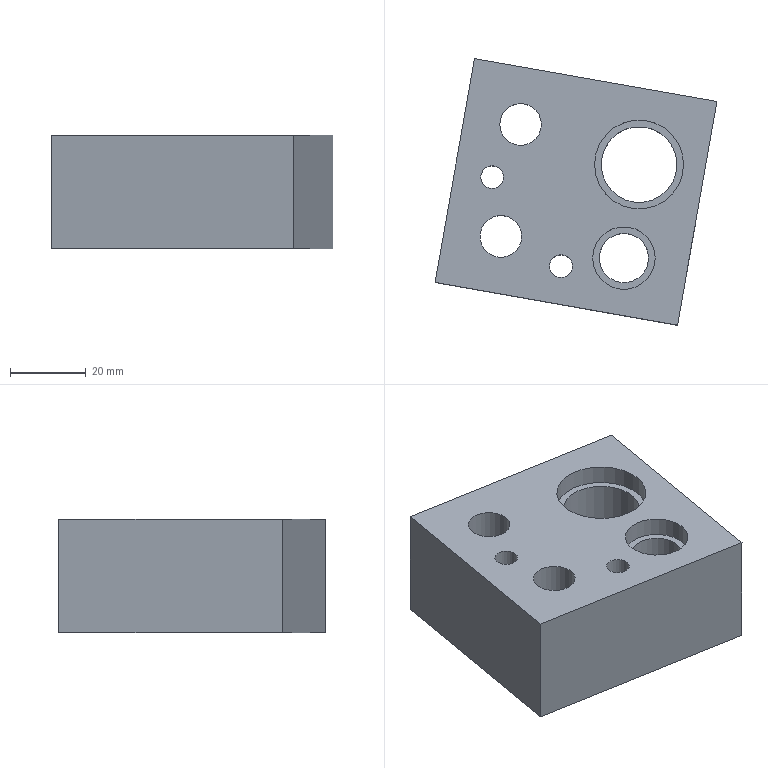Part | NX | features solid 2 | 1 solid | 20 faces | box 74.431 x 70.376 x 30 mm | volume 92025 mm3 | plane 10 | cylinder 10 | commonest cylinder face diameters 6 x2 11 x2 17 x2 13 x1 16.5 x1 20 x1
STEP:
#1=CARTESIAN_POINT('',(471.302,165.949,33.192));
#2=VERTEX_POINT('',#1);
#3=CARTESIAN_POINT('',(461.302,165.949,33.192));
#4=DIRECTION('',(0.000000502,0.000000149,1.));
#5=DIRECTION('',(1.,-0.000001668,-0.000000502));
#6=AXIS2_PLACEMENT_3D('',#3,#4,#5);
#7=CIRCLE('',#6,10.);
#8=EDGE_CURVE('',#2,#2,#7,.F.);
#9=ORIENTED_EDGE('',*,*,#8,.F.);
#10=EDGE_LOOP('',(#9));
#11=FACE_BOUND('',#10,.T.);
#12=CARTESIAN_POINT('',(416.303,147.002,33.192));
#13=VERTEX_POINT('',#12);
#14=CARTESIAN_POINT('',(424.803,147.002,33.192));
#15=DIRECTION('',(-0.000000502,-0.000000149,-1.));
#16=DIRECTION('',(-1.,0.000001668,0.000000502));
#17=AXIS2_PLACEMENT_3D('',#14,#15,#16);
#18=CIRCLE('',#17,8.5);
#19=EDGE_CURVE('',#13,#13,#18,.T.);
#20=ORIENTED_EDGE('',*,*,#19,.F.);
#21=EDGE_LOOP('',(#20));
#22=FACE_BOUND('',#21,.T.);
#23=CARTESIAN_POINT('',(421.512,176.546,33.192));
#24=VERTEX_POINT('',#23);
#25=CARTESIAN_POINT('',(430.012,176.546,33.192));
#26=DIRECTION('',(-0.000000502,-0.000000149,-1.));
#27=DIRECTION('',(-1.,0.000001668,0.000000502));
#28=AXIS2_PLACEMENT_3D('',#25,#26,#27);
#29=CIRCLE('',#28,8.5);
#30=EDGE_CURVE('',#24,#24,#29,.T.);
#31=ORIENTED_EDGE('',*,*,#30,.F.);
#32=EDGE_LOOP('',(#31));
#33=FACE_BOUND('',#32,.T.);
#34=CARTESIAN_POINT('',(407.426,134.834,33.192));
#35=VERTEX_POINT('',#34);
#36=CARTESIAN_POINT('',(417.845,193.923,33.192));
#37=VERTEX_POINT('',#36);
#38=CARTESIAN_POINT('',(418.713,198.847,33.192));
#39=DIRECTION('',(0.1736,0.9848,-0.000000234));
#40=VECTOR('',#39,1000.);
#41=LINE('',#38,#40);
#42=EDGE_CURVE('',#35,#37,#41,.T.);
#43=ORIENTED_EDGE('',*,*,#42,.T.);
#44=CARTESIAN_POINT('',(481.857,182.635,33.192));
#45=VERTEX_POINT('',#44);
#46=CARTESIAN_POINT('',(415.875,194.27,33.192));
#47=DIRECTION('',(0.9848,-0.1736,-0.000000468));
#48=VECTOR('',#47,1000.);
#49=LINE('',#46,#48);
#50=EDGE_CURVE('',#37,#45,#49,.T.);
#51=ORIENTED_EDGE('',*,*,#50,.T.);
#52=CARTESIAN_POINT('',(471.438,123.547,33.192));
#53=VERTEX_POINT('',#52);
#54=CARTESIAN_POINT('',(482.726,187.559,33.192));
#55=DIRECTION('',(-0.1736,-0.9848,0.000000234));
#56=VECTOR('',#55,1000.);
#57=LINE('',#54,#56);
#58=EDGE_CURVE('',#45,#53,#57,.T.);
#59=ORIENTED_EDGE('',*,*,#58,.T.);
#60=CARTESIAN_POINT('',(405.456,135.181,33.192));
#61=DIRECTION('',(-0.9848,0.1736,0.000000468));
#62=VECTOR('',#61,1000.);
#63=LINE('',#60,#62);
#64=EDGE_CURVE('',#53,#35,#63,.T.);
#65=ORIENTED_EDGE('',*,*,#64,.T.);
#66=EDGE_LOOP('',(#43,#51,#59,#65));
#67=FACE_BOUND('',#66,.T.);
#68=CARTESIAN_POINT('',(463.801,141.271,33.192));
#69=VERTEX_POINT('',#68);
#70=CARTESIAN_POINT('',(457.301,141.271,33.192));
#71=DIRECTION('',(0.000000502,0.000000149,1.));
#72=DIRECTION('',(1.,-0.000001668,-0.000000502));
#73=AXIS2_PLACEMENT_3D('',#70,#71,#72);
#74=CIRCLE('',#73,6.5);
#75=EDGE_CURVE('',#69,#69,#74,.F.);
#76=ORIENTED_EDGE('',*,*,#75,.F.);
#77=EDGE_LOOP('',(#76));
#78=FACE_BOUND('',#77,.T.);
#79=CARTESIAN_POINT('',(425.484,162.642,33.192));
#80=VERTEX_POINT('',#79);
#81=CARTESIAN_POINT('',(422.484,162.642,33.192));
#82=DIRECTION('',(0.000000502,0.000000149,1.));
#83=DIRECTION('',(1.,0.,-0.000000502));
#84=AXIS2_PLACEMENT_3D('',#81,#82,#83);
#85=CIRCLE('',#84,3.);
#86=EDGE_CURVE('',#80,#80,#85,.F.);
#87=ORIENTED_EDGE('',*,*,#86,.F.);
#88=EDGE_LOOP('',(#87));
#89=FACE_BOUND('',#88,.T.);
#90=CARTESIAN_POINT('',(443.676,139.125,33.192));
#91=VERTEX_POINT('',#90);
#92=CARTESIAN_POINT('',(440.676,139.125,33.192));
#93=DIRECTION('',(0.000000502,0.000000149,1.));
#94=DIRECTION('',(1.,0.,-0.000000502));
#95=AXIS2_PLACEMENT_3D('',#92,#93,#94);
#96=CIRCLE('',#95,3.);
#97=EDGE_CURVE('',#91,#91,#96,.F.);
#98=ORIENTED_EDGE('',*,*,#97,.F.);
#99=EDGE_LOOP('',(#98));
#100=FACE_BOUND('',#99,.T.);
#101=CARTESIAN_POINT('',(416.744,199.194,33.192));
#102=DIRECTION('',(-0.000000502,-0.000000149,-1.));
#103=DIRECTION('',(0.9848,-0.1736,-0.000000468));
#104=AXIS2_PLACEMENT_3D('',#101,#102,#103);
#105=PLANE('',#104);
#106=ADVANCED_FACE('',(#11,#22,#33,#67,#78,#89,#100),#105,.T.);
#107=CARTESIAN_POINT('',(443.676,139.125,63.192));
#108=VERTEX_POINT('',#107);
#109=CARTESIAN_POINT('',(440.676,139.125,63.192));
#110=DIRECTION('',(0.000000502,0.000000149,1.));
#111=DIRECTION('',(1.,-0.000001668,-0.000000502));
#112=AXIS2_PLACEMENT_3D('',#109,#110,#111);
#113=CIRCLE('',#112,3.);
#114=EDGE_CURVE('',#108,#108,#113,.F.);
#115=ORIENTED_EDGE('',*,*,#114,.T.);
#116=EDGE_LOOP('',(#115));
#117=FACE_BOUND('',#116,.T.);
#118=CARTESIAN_POINT('',(425.484,162.642,63.192));
#119=VERTEX_POINT('',#118);
#120=CARTESIAN_POINT('',(422.484,162.642,63.192));
#121=DIRECTION('',(0.000000502,0.000000149,1.));
#122=DIRECTION('',(1.,-0.000001668,-0.000000502));
#123=AXIS2_PLACEMENT_3D('',#120,#121,#122);
#124=CIRCLE('',#123,3.);
#125=EDGE_CURVE('',#119,#119,#124,.F.);
#126=ORIENTED_EDGE('',*,*,#125,.T.);
#127=EDGE_LOOP('',(#126));
#128=FACE_BOUND('',#127,.T.);
#129=CARTESIAN_POINT('',(473.052,165.949,63.192));
#130=VERTEX_POINT('',#129);
#131=CARTESIAN_POINT('',(461.302,165.949,63.192));
#132=DIRECTION('',(0.000000502,0.000000149,1.));
#133=DIRECTION('',(1.,-0.000001668,-0.000000502));
#134=AXIS2_PLACEMENT_3D('',#131,#132,#133);
#135=CIRCLE('',#134,11.75);
#136=EDGE_CURVE('',#130,#130,#135,.T.);
#137=ORIENTED_EDGE('',*,*,#136,.F.);
#138=EDGE_LOOP('',(#137));
#139=FACE_BOUND('',#138,.T.);
#140=CARTESIAN_POINT('',(430.303,147.002,63.192));
#141=VERTEX_POINT('',#140);
#142=CARTESIAN_POINT('',(424.803,147.002,63.192));
#143=DIRECTION('',(0.000000502,0.000000149,1.));
#144=DIRECTION('',(1.,-0.000001668,-0.000000502));
#145=AXIS2_PLACEMENT_3D('',#142,#143,#144);
#146=CIRCLE('',#145,5.5);
#147=EDGE_CURVE('',#141,#141,#146,.F.);
#148=ORIENTED_EDGE('',*,*,#147,.T.);
#149=EDGE_LOOP('',(#148));
#150=FACE_BOUND('',#149,.T.);
#151=CARTESIAN_POINT('',(435.512,176.546,63.192));
#152=VERTEX_POINT('',#151);
#153=CARTESIAN_POINT('',(430.012,176.546,63.192));
#154=DIRECTION('',(0.000000502,0.000000149,1.));
#155=DIRECTION('',(1.,-0.000001668,-0.000000502));
#156=AXIS2_PLACEMENT_3D('',#153,#154,#155);
#157=CIRCLE('',#156,5.5);
#158=EDGE_CURVE('',#152,#152,#157,.F.);
#159=ORIENTED_EDGE('',*,*,#158,.T.);
#160=EDGE_LOOP('',(#159));
#161=FACE_BOUND('',#160,.T.);
#162=CARTESIAN_POINT('',(407.426,134.834,63.192));
#163=VERTEX_POINT('',#162);
#164=CARTESIAN_POINT('',(471.438,123.547,63.192));
#165=VERTEX_POINT('',#164);
#166=CARTESIAN_POINT('',(405.456,135.181,63.192));
#167=DIRECTION('',(-0.9848,0.1736,0.000000468));
#168=VECTOR('',#167,1000.);
#169=LINE('',#166,#168);
#170=EDGE_CURVE('',#163,#165,#169,.F.);
#171=ORIENTED_EDGE('',*,*,#170,.T.);
#172=CARTESIAN_POINT('',(481.857,182.635,63.192));
#173=VERTEX_POINT('',#172);
#174=CARTESIAN_POINT('',(482.726,187.559,63.192));
#175=DIRECTION('',(-0.1736,-0.9848,0.000000234));
#176=VECTOR('',#175,1000.);
#177=LINE('',#174,#176);
#178=EDGE_CURVE('',#165,#173,#177,.F.);
#179=ORIENTED_EDGE('',*,*,#178,.T.);
#180=CARTESIAN_POINT('',(417.845,193.923,63.192));
#181=VERTEX_POINT('',#180);
#182=CARTESIAN_POINT('',(415.875,194.27,63.192));
#183=DIRECTION('',(0.9848,-0.1736,-0.000000468));
#184=VECTOR('',#183,1000.);
#185=LINE('',#182,#184);
#186=EDGE_CURVE('',#173,#181,#185,.F.);
#187=ORIENTED_EDGE('',*,*,#186,.T.);
#188=CARTESIAN_POINT('',(418.713,198.847,63.192));
#189=DIRECTION('',(0.1736,0.9848,-0.000000234));
#190=VECTOR('',#189,1000.);
#191=LINE('',#188,#190);
#192=EDGE_CURVE('',#181,#163,#191,.F.);
#193=ORIENTED_EDGE('',*,*,#192,.T.);
#194=EDGE_LOOP('',(#171,#179,#187,#193));
#195=FACE_BOUND('',#194,.T.);
#196=CARTESIAN_POINT('',(465.551,141.271,63.192));
#197=VERTEX_POINT('',#196);
#198=CARTESIAN_POINT('',(457.301,141.271,63.192));
#199=DIRECTION('',(0.000000502,0.000000149,1.));
#200=DIRECTION('',(1.,-0.000001668,-0.000000502));
#201=AXIS2_PLACEMENT_3D('',#198,#199,#200);
#202=CIRCLE('',#201,8.25);
#203=EDGE_CURVE('',#197,#197,#202,.T.);
#204=ORIENTED_EDGE('',*,*,#203,.F.);
#205=EDGE_LOOP('',(#204));
#206=FACE_BOUND('',#205,.T.);
#207=CARTESIAN_POINT('',(486.873,147.734,63.192));
#208=DIRECTION('',(-0.000000502,-0.000000149,-1.));
#209=DIRECTION('',(0.9848,-0.1736,-0.000000468));
#210=AXIS2_PLACEMENT_3D('',#207,#208,#209);
#211=PLANE('',#210);
#212=ADVANCED_FACE('',(#117,#128,#139,#150,#161,#195,#206),#211,.F.);
#213=CARTESIAN_POINT('',(407.426,134.834,63.192));
#214=DIRECTION('',(0.000000502,0.000000149,1.));
#215=VECTOR('',#214,1000.);
#216=LINE('',#213,#215);
#217=EDGE_CURVE('',#35,#163,#216,.T.);
#218=ORIENTED_EDGE('',*,*,#217,.F.);
#219=ORIENTED_EDGE('',*,*,#64,.F.);
#220=CARTESIAN_POINT('',(471.438,123.547,63.192));
#221=DIRECTION('',(0.000000502,0.000000149,1.));
#222=VECTOR('',#221,1000.);
#223=LINE('',#220,#222);
#224=EDGE_CURVE('',#53,#165,#223,.T.);
#225=ORIENTED_EDGE('',*,*,#224,.T.);
#226=ORIENTED_EDGE('',*,*,#170,.F.);
#227=EDGE_LOOP('',(#218,#219,#225,#226));
#228=FACE_BOUND('',#227,.T.);
#229=CARTESIAN_POINT('',(405.456,135.181,63.192));
#230=DIRECTION('',(-0.1736,-0.9848,0.000000234));
#231=DIRECTION('',(-0.000000502,-0.000000149,-1.));
#232=AXIS2_PLACEMENT_3D('',#229,#230,#231);
#233=PLANE('',#232);
#234=ADVANCED_FACE('',(#228),#233,.T.);
#235=ORIENTED_EDGE('',*,*,#224,.F.);
#236=ORIENTED_EDGE('',*,*,#58,.F.);
#237=CARTESIAN_POINT('',(481.857,182.635,63.192));
#238=DIRECTION('',(0.000000502,0.000000149,1.));
#239=VECTOR('',#238,1000.);
#240=LINE('',#237,#239);
#241=EDGE_CURVE('',#45,#173,#240,.T.);
#242=ORIENTED_EDGE('',*,*,#241,.T.);
#243=ORIENTED_EDGE('',*,*,#178,.F.);
#244=EDGE_LOOP('',(#235,#236,#242,#243));
#245=FACE_BOUND('',#244,.T.);
#246=CARTESIAN_POINT('',(482.726,187.559,63.192));
#247=DIRECTION('',(0.9848,-0.1736,-0.000000468));
#248=DIRECTION('',(0.000000502,0.000000149,1.));
#249=AXIS2_PLACEMENT_3D('',#246,#247,#248);
#250=PLANE('',#249);
#251=ADVANCED_FACE('',(#245),#250,.T.);
#252=ORIENTED_EDGE('',*,*,#241,.F.);
#253=ORIENTED_EDGE('',*,*,#50,.F.);
#254=CARTESIAN_POINT('',(417.845,193.923,63.192));
#255=DIRECTION('',(0.000000502,0.000000149,1.));
#256=VECTOR('',#255,1000.);
#257=LINE('',#254,#256);
#258=EDGE_CURVE('',#37,#181,#257,.T.);
#259=ORIENTED_EDGE('',*,*,#258,.T.);
#260=ORIENTED_EDGE('',*,*,#186,.F.);
#261=EDGE_LOOP('',(#252,#253,#259,#260));
#262=FACE_BOUND('',#261,.T.);
#263=CARTESIAN_POINT('',(415.875,194.27,63.192));
#264=DIRECTION('',(0.1736,0.9848,-0.000000234));
#265=DIRECTION('',(0.000000502,0.000000149,1.));
#266=AXIS2_PLACEMENT_3D('',#263,#264,#265);
#267=PLANE('',#266);
#268=ADVANCED_FACE('',(#262),#267,.T.);
#269=ORIENTED_EDGE('',*,*,#42,.F.);
#270=ORIENTED_EDGE('',*,*,#217,.T.);
#271=ORIENTED_EDGE('',*,*,#192,.F.);
#272=ORIENTED_EDGE('',*,*,#258,.F.);
#273=EDGE_LOOP('',(#269,#270,#271,#272));
#274=FACE_BOUND('',#273,.T.);
#275=CARTESIAN_POINT('',(418.713,198.847,63.192));
#276=DIRECTION('',(-0.9848,0.1736,0.000000468));
#277=DIRECTION('',(-0.000000502,-0.000000149,-1.));
#278=AXIS2_PLACEMENT_3D('',#275,#276,#277);
#279=PLANE('',#278);
#280=ADVANCED_FACE('',(#274),#279,.T.);
#281=ORIENTED_EDGE('',*,*,#158,.F.);
#282=EDGE_LOOP('',(#281));
#283=FACE_BOUND('',#282,.T.);
#284=CARTESIAN_POINT('',(424.512,176.546,45.192));
#285=VERTEX_POINT('',#284);
#286=CARTESIAN_POINT('',(430.012,176.546,45.192));
#287=DIRECTION('',(-0.000000502,-0.000000149,-1.));
#288=DIRECTION('',(-1.,0.000001668,0.000000502));
#289=AXIS2_PLACEMENT_3D('',#286,#287,#288);
#290=CIRCLE('',#289,5.5);
#291=EDGE_CURVE('',#285,#285,#290,.T.);
#292=ORIENTED_EDGE('',*,*,#291,.T.);
#293=EDGE_LOOP('',(#292));
#294=FACE_BOUND('',#293,.T.);
#295=CARTESIAN_POINT('',(430.012,176.546,83.192));
#296=DIRECTION('',(0.000000502,0.000000149,1.));
#297=DIRECTION('',(-1.,0.000001668,0.000000502));
#298=AXIS2_PLACEMENT_3D('',#295,#296,#297);
#299=CYLINDRICAL_SURFACE('',#298,5.5);
#300=ADVANCED_FACE('',(#283,#294),#299,.F.);
#301=ORIENTED_EDGE('',*,*,#291,.F.);
#302=EDGE_LOOP('',(#301));
#303=FACE_BOUND('',#302,.T.);
#304=CARTESIAN_POINT('',(421.512,176.546,45.192));
#305=VERTEX_POINT('',#304);
#306=CARTESIAN_POINT('',(430.012,176.546,45.192));
#307=DIRECTION('',(-0.000000502,-0.000000149,-1.));
#308=DIRECTION('',(-1.,0.000001668,0.000000502));
#309=AXIS2_PLACEMENT_3D('',#306,#307,#308);
#310=CIRCLE('',#309,8.5);
#311=EDGE_CURVE('',#305,#305,#310,.T.);
#312=ORIENTED_EDGE('',*,*,#311,.T.);
#313=EDGE_LOOP('',(#312));
#314=FACE_BOUND('',#313,.T.);
#315=CARTESIAN_POINT('',(430.012,176.546,45.192));
#316=DIRECTION('',(0.000000502,0.000000149,1.));
#317=DIRECTION('',(-1.,0.000001668,0.000000502));
#318=AXIS2_PLACEMENT_3D('',#315,#316,#317);
#319=PLANE('',#318);
#320=ADVANCED_FACE('',(#303,#314),#319,.F.);
#321=ORIENTED_EDGE('',*,*,#311,.F.);
#322=EDGE_LOOP('',(#321));
#323=FACE_BOUND('',#322,.T.);
#324=ORIENTED_EDGE('',*,*,#30,.T.);
#325=EDGE_LOOP('',(#324));
#326=FACE_BOUND('',#325,.T.);
#327=CARTESIAN_POINT('',(430.012,176.546,33.192));
#328=DIRECTION('',(0.000000502,0.000000149,1.));
#329=DIRECTION('',(-1.,0.000001668,0.000000502));
#330=AXIS2_PLACEMENT_3D('',#327,#328,#329);
#331=CYLINDRICAL_SURFACE('',#330,8.5);
#332=ADVANCED_FACE('',(#323,#326),#331,.F.);
#333=ORIENTED_EDGE('',*,*,#147,.F.);
#334=EDGE_LOOP('',(#333));
#335=FACE_BOUND('',#334,.T.);
#336=CARTESIAN_POINT('',(419.303,147.002,45.192));
#337=VERTEX_POINT('',#336);
#338=CARTESIAN_POINT('',(424.803,147.002,45.192));
#339=DIRECTION('',(-0.000000502,-0.000000149,-1.));
#340=DIRECTION('',(-1.,0.000001668,0.000000502));
#341=AXIS2_PLACEMENT_3D('',#338,#339,#340);
#342=CIRCLE('',#341,5.5);
#343=EDGE_CURVE('',#337,#337,#342,.T.);
#344=ORIENTED_EDGE('',*,*,#343,.T.);
#345=EDGE_LOOP('',(#344));
#346=FACE_BOUND('',#345,.T.);
#347=CARTESIAN_POINT('',(424.803,147.002,83.192));
#348=DIRECTION('',(0.000000502,0.000000149,1.));
#349=DIRECTION('',(-1.,0.000001668,0.000000502));
#350=AXIS2_PLACEMENT_3D('',#347,#348,#349);
#351=CYLINDRICAL_SURFACE('',#350,5.5);
#352=ADVANCED_FACE('',(#335,#346),#351,.F.);
#353=ORIENTED_EDGE('',*,*,#343,.F.);
#354=EDGE_LOOP('',(#353));
#355=FACE_BOUND('',#354,.T.);
#356=CARTESIAN_POINT('',(416.303,147.002,45.192));
#357=VERTEX_POINT('',#356);
#358=CARTESIAN_POINT('',(424.803,147.002,45.192));
#359=DIRECTION('',(-0.000000502,-0.000000149,-1.));
#360=DIRECTION('',(-1.,0.000001668,0.000000502));
#361=AXIS2_PLACEMENT_3D('',#358,#359,#360);
#362=CIRCLE('',#361,8.5);
#363=EDGE_CURVE('',#357,#357,#362,.T.);
#364=ORIENTED_EDGE('',*,*,#363,.T.);
#365=EDGE_LOOP('',(#364));
#366=FACE_BOUND('',#365,.T.);
#367=CARTESIAN_POINT('',(424.803,147.002,45.192));
#368=DIRECTION('',(0.000000502,0.000000149,1.));
#369=DIRECTION('',(-1.,0.000001668,0.000000502));
#370=AXIS2_PLACEMENT_3D('',#367,#368,#369);
#371=PLANE('',#370);
#372=ADVANCED_FACE('',(#355,#366),#371,.F.);
#373=ORIENTED_EDGE('',*,*,#363,.F.);
#374=EDGE_LOOP('',(#373));
#375=FACE_BOUND('',#374,.T.);
#376=ORIENTED_EDGE('',*,*,#19,.T.);
#377=EDGE_LOOP('',(#376));
#378=FACE_BOUND('',#377,.T.);
#379=CARTESIAN_POINT('',(424.803,147.002,33.192));
#380=DIRECTION('',(0.000000502,0.000000149,1.));
#381=DIRECTION('',(-1.,0.000001668,0.000000502));
#382=AXIS2_PLACEMENT_3D('',#379,#380,#381);
#383=CYLINDRICAL_SURFACE('',#382,8.5);
#384=ADVANCED_FACE('',(#375,#378),#383,.F.);
#385=ORIENTED_EDGE('',*,*,#136,.T.);
#386=EDGE_LOOP('',(#385));
#387=FACE_BOUND('',#386,.T.);
#388=CARTESIAN_POINT('',(449.552,165.949,58.192));
#389=VERTEX_POINT('',#388);
#390=CARTESIAN_POINT('',(461.302,165.949,58.192));
#391=DIRECTION('',(0.000000502,0.000000149,1.));
#392=DIRECTION('',(-1.,0.000001668,0.000000502));
#393=AXIS2_PLACEMENT_3D('',#390,#391,#392);
#394=CIRCLE('',#393,11.75);
#395=EDGE_CURVE('',#389,#389,#394,.T.);
#396=ORIENTED_EDGE('',*,*,#395,.F.);
#397=EDGE_LOOP('',(#396));
#398=FACE_BOUND('',#397,.T.);
#399=CARTESIAN_POINT('',(461.302,165.949,58.192));
#400=DIRECTION('',(0.000000502,0.000000149,1.));
#401=DIRECTION('',(-1.,0.000001668,0.000000502));
#402=AXIS2_PLACEMENT_3D('',#399,#400,#401);
#403=CYLINDRICAL_SURFACE('',#402,11.75);
#404=ADVANCED_FACE('',(#387,#398),#403,.F.);
#405=ORIENTED_EDGE('',*,*,#395,.T.);
#406=EDGE_LOOP('',(#405));
#407=FACE_BOUND('',#406,.T.);
#408=CARTESIAN_POINT('',(471.302,165.949,58.192));
#409=VERTEX_POINT('',#408);
#410=CARTESIAN_POINT('',(461.302,165.949,58.192));
#411=DIRECTION('',(-0.000000502,-0.000000149,-1.));
#412=DIRECTION('',(1.,-0.000001668,-0.000000502));
#413=AXIS2_PLACEMENT_3D('',#410,#411,#412);
#414=CIRCLE('',#413,10.);
#415=EDGE_CURVE('',#409,#409,#414,.T.);
#416=ORIENTED_EDGE('',*,*,#415,.T.);
#417=EDGE_LOOP('',(#416));
#418=FACE_BOUND('',#417,.T.);
#419=CARTESIAN_POINT('',(461.302,165.949,58.192));
#420=DIRECTION('',(-0.000000502,-0.000000149,-1.));
#421=DIRECTION('',(1.,-0.000001668,-0.000000502));
#422=AXIS2_PLACEMENT_3D('',#419,#420,#421);
#423=PLANE('',#422);
#424=ADVANCED_FACE('',(#407,#418),#423,.F.);
#425=ORIENTED_EDGE('',*,*,#203,.T.);
#426=EDGE_LOOP('',(#425));
#427=FACE_BOUND('',#426,.T.);
#428=CARTESIAN_POINT('',(465.551,141.271,58.192));
#429=VERTEX_POINT('',#428);
#430=CARTESIAN_POINT('',(457.301,141.271,58.192));
#431=DIRECTION('',(0.000000502,0.000000149,1.));
#432=DIRECTION('',(1.,-0.000001668,-0.000000502));
#433=AXIS2_PLACEMENT_3D('',#430,#431,#432);
#434=CIRCLE('',#433,8.25);
#435=EDGE_CURVE('',#429,#429,#434,.T.);
#436=ORIENTED_EDGE('',*,*,#435,.F.);
#437=EDGE_LOOP('',(#436));
#438=FACE_BOUND('',#437,.T.);
#439=CARTESIAN_POINT('',(457.301,141.271,58.192));
#440=DIRECTION('',(0.000000502,0.000000149,1.));
#441=DIRECTION('',(-1.,0.000001668,0.000000502));
#442=AXIS2_PLACEMENT_3D('',#439,#440,#441);
#443=CYLINDRICAL_SURFACE('',#442,8.25);
#444=ADVANCED_FACE('',(#427,#438),#443,.F.);
#445=ORIENTED_EDGE('',*,*,#435,.T.);
#446=EDGE_LOOP('',(#445));
#447=FACE_BOUND('',#446,.T.);
#448=CARTESIAN_POINT('',(450.801,141.271,58.192));
#449=VERTEX_POINT('',#448);
#450=CARTESIAN_POINT('',(457.301,141.271,58.192));
#451=DIRECTION('',(-0.000000502,-0.000000149,-1.));
#452=DIRECTION('',(-1.,0.000001668,0.000000502));
#453=AXIS2_PLACEMENT_3D('',#450,#451,#452);
#454=CIRCLE('',#453,6.5);
#455=EDGE_CURVE('',#449,#449,#454,.T.);
#456=ORIENTED_EDGE('',*,*,#455,.T.);
#457=EDGE_LOOP('',(#456));
#458=FACE_BOUND('',#457,.T.);
#459=CARTESIAN_POINT('',(457.301,141.271,58.192));
#460=DIRECTION('',(-0.000000502,-0.000000149,-1.));
#461=DIRECTION('',(1.,-0.000001668,-0.000000502));
#462=AXIS2_PLACEMENT_3D('',#459,#460,#461);
#463=PLANE('',#462);
#464=ADVANCED_FACE('',(#447,#458),#463,.F.);
#465=ORIENTED_EDGE('',*,*,#8,.T.);
#466=EDGE_LOOP('',(#465));
#467=FACE_BOUND('',#466,.T.);
#468=ORIENTED_EDGE('',*,*,#415,.F.);
#469=EDGE_LOOP('',(#468));
#470=FACE_BOUND('',#469,.T.);
#471=CARTESIAN_POINT('',(461.302,165.949,63.192));
#472=DIRECTION('',(-0.000000502,-0.000000149,-1.));
#473=DIRECTION('',(-1.,0.000001668,0.000000502));
#474=AXIS2_PLACEMENT_3D('',#471,#472,#473);
#475=CYLINDRICAL_SURFACE('',#474,10.);
#476=ADVANCED_FACE('',(#467,#470),#475,.F.);
#477=ORIENTED_EDGE('',*,*,#75,.T.);
#478=EDGE_LOOP('',(#477));
#479=FACE_BOUND('',#478,.T.);
#480=ORIENTED_EDGE('',*,*,#455,.F.);
#481=EDGE_LOOP('',(#480));
#482=FACE_BOUND('',#481,.T.);
#483=CARTESIAN_POINT('',(457.301,141.271,63.192));
#484=DIRECTION('',(-0.000000502,-0.000000149,-1.));
#485=DIRECTION('',(1.,-0.000001668,-0.000000502));
#486=AXIS2_PLACEMENT_3D('',#483,#484,#485);
#487=CYLINDRICAL_SURFACE('',#486,6.5);
#488=ADVANCED_FACE('',(#479,#482),#487,.F.);
#489=ORIENTED_EDGE('',*,*,#125,.F.);
#490=EDGE_LOOP('',(#489));
#491=FACE_BOUND('',#490,.T.);
#492=ORIENTED_EDGE('',*,*,#86,.T.);
#493=EDGE_LOOP('',(#492));
#494=FACE_BOUND('',#493,.T.);
#495=CARTESIAN_POINT('',(422.484,162.642,83.192));
#496=DIRECTION('',(0.000000502,0.000000149,1.));
#497=DIRECTION('',(-1.,0.000001668,0.000000502));
#498=AXIS2_PLACEMENT_3D('',#495,#496,#497);
#499=CYLINDRICAL_SURFACE('',#498,3.);
#500=ADVANCED_FACE('',(#491,#494),#499,.F.);
#501=ORIENTED_EDGE('',*,*,#114,.F.);
#502=EDGE_LOOP('',(#501));
#503=FACE_BOUND('',#502,.T.);
#504=ORIENTED_EDGE('',*,*,#97,.T.);
#505=EDGE_LOOP('',(#504));
#506=FACE_BOUND('',#505,.T.);
#507=CARTESIAN_POINT('',(440.676,139.125,83.192));
#508=DIRECTION('',(0.000000502,0.000000149,1.));
#509=DIRECTION('',(-1.,0.000001668,0.000000502));
#510=AXIS2_PLACEMENT_3D('',#507,#508,#509);
#511=CYLINDRICAL_SURFACE('',#510,3.);
#512=ADVANCED_FACE('',(#503,#506),#511,.F.);
#513=CLOSED_SHELL('',(#106,#212,#234,#251,#268,#280,#300,#320,#332,#352,#372,#384,#404,#424,#444,#464,#476,#488,#500,#512));
#514=MANIFOLD_SOLID_BREP('',#513);
#515=(LENGTH_UNIT()NAMED_UNIT(*)SI_UNIT(.MILLI.,.METRE.));
#516=UNCERTAINTY_MEASURE_WITH_UNIT(LENGTH_MEASURE(0.00001),#515,'','');
#517=(NAMED_UNIT(*)PLANE_ANGLE_UNIT()SI_UNIT($,.RADIAN.));
#518=(NAMED_UNIT(*)SI_UNIT($,.STERADIAN.)SOLID_ANGLE_UNIT());
#519=(GEOMETRIC_REPRESENTATION_CONTEXT(3)GLOBAL_UNCERTAINTY_ASSIGNED_CONTEXT((#516))GLOBAL_UNIT_ASSIGNED_CONTEXT((#515,#517,#518))REPRESENTATION_CONTEXT('',''));
#520=ADVANCED_BREP_SHAPE_REPRESENTATION('',(#514),#519);